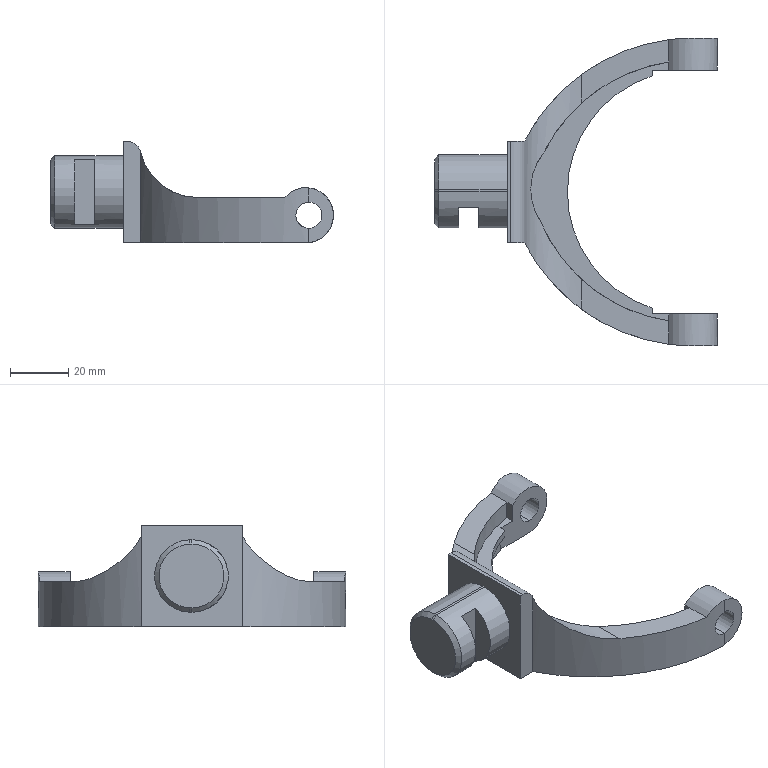Part | SolidWorks | features BaseBody 1 | 1 solid | 47 faces | box 97.5 x 106 x 35 mm | volume 48605 mm3 | plane 25 | cylinder 20 | cone 2 | commonest cylinder face diameters 9 x4 40 x3 19 x2 84 x2 87.818 x2 130 x2